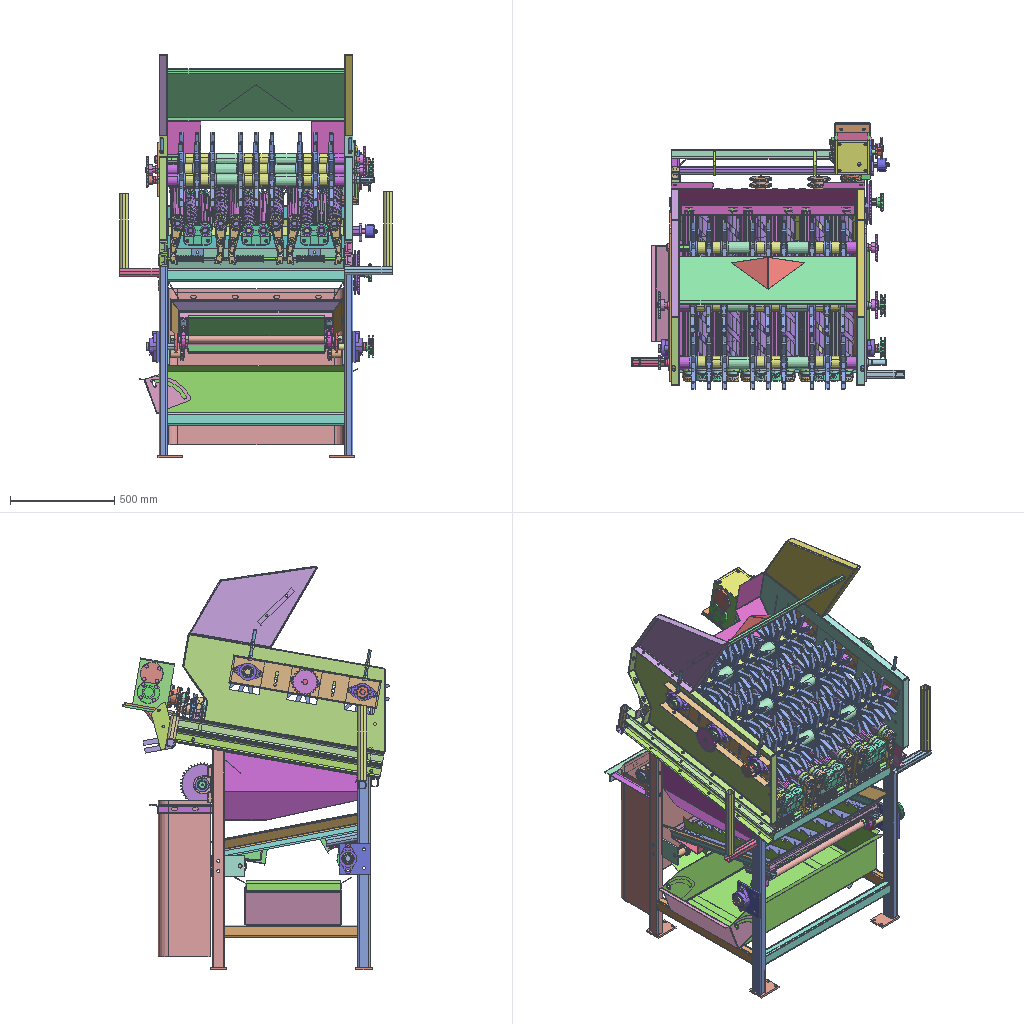Assembly | SolidWorks | 205 different items | 650 placed | box 1308 x 1283 x 1941 mm
Parts list (item | name | quantity | parent item | size | volume | features):
1 | (subassembly) | x2 | - | 262.006 x 262.006 x 1096 mm | 5906845 mm3 | features LayoutProfileFeature 1
2 | (subassembly) | x1 | in 3 | 32 x 32 x 1016 mm | 377179 mm3 | features LayoutProfileFeature 1
3 | (subassembly) | x1 | - | 262.006 x 262.006 x 1016 mm | 5789700 mm3 | features LayoutProfileFeature 1
4 | (subassembly) | x1 | - | 829.179 x 774.462 x 164.679 mm | 3231885 mm3 | features LayoutProfileFeature 1
5 | (subassembly) | x1 | in 6 | 1308 x 1116 x 1270 mm | 7450780 mm3 | features LayoutProfileFeature 1
6 | (subassembly) | x1 | - | 1308 x 1116 x 1280 mm | 8216576 mm3 | features LayoutProfileFeature 1
7 | (subassembly) | x1 | - | 1011 x 975.086 x 897.064 mm | 6794534 mm3 | features LayoutProfileFeature 1
8 | (subassembly) | x1 | in 7 | 852 x 259.795 x 223.71 mm | 531072 mm3 | features LayoutProfileFeature 1
9 | (subassembly) | x1 | - | - | 51530295 mm3 | features LayoutProfileFeature 1
10 | (subassembly) | x2 | in 7 | 136 x 720 x 55.5 mm | 917800 mm3 | features LayoutProfileFeature 1
11 | (subassembly) | x1 | in 43 | 5 x 8 x 18 mm | 644.24 mm3 | features LayoutProfileFeature 1
12 | (subassembly) | x1 | - | 95 x 60 x 141 mm | 156378 mm3 | features LayoutProfileFeature 1
13 | (subassembly) | x1 | - | 1048 x 561.923 x 252.092 mm | 2371643 mm3 | features LayoutProfileFeature 1
14 | (subassembly) | x2 | - | 171 x 100 x 85 mm | 236433 mm3 | features LayoutProfileFeature 1
15 | (subassembly) | x1 | in 24 | 680 x 740 x 40 mm | 649422 mm3 | features LayoutProfileFeature 1
16 | (subassembly) | x2 | in 1 | 32 x 32.7 x 1096 mm | 415799 mm3 | features LayoutProfileFeature 1
17 | (subassembly) | x1 | in 9 | 257.243 x 1277 x 974 mm | 4686993 mm3 | features LayoutProfileFeature 1
18 | (subassembly) | x2 | in 19 | 37 x 50 x 50 mm | 36117 mm3 | features LayoutProfileFeature 1
19 | (subassembly) | x1 | in 17 | 257.243 x 1277 x 974 mm | 4686993 mm3 | features LayoutProfileFeature 1
20 | (subassembly) | x6 | in 36 | - | 16373 mm3 | features LayoutProfileFeature 1
21 | (subassembly) | x12 | in 26, 30 | 60 x 226.322 x 40 mm | 177077 mm3 | features LayoutProfileFeature 1
22 | (subassembly) | x1 | in 43 | 5 x 8 x 18 mm | 644.24 mm3 | features LayoutProfileFeature 1
23 | (subassembly) | x2 | in 4 | 40 x 40 x 185 mm | 91393 mm3 | features LayoutProfileFeature 1
24 | (subassembly) | x1 | in 4 | 829.179 x 774.462 x 88.771 mm | 2637561 mm3 | features LayoutProfileFeature 1
25 | (subassembly) | x1 | - | 86.409 x 82.969 x 184 mm | 179233 mm3 | features LayoutProfileFeature 1
26 | (subassembly) | x3 | in 9 | 934.5 x 236.345 x 93.958 mm | 3556008 mm3 | features LayoutProfileFeature 1
27 | (subassembly) | x1 | in 5 | 932 x 40 x 300 mm | 437603 mm3 | features LayoutProfileFeature 1
28 | (subassembly) | x6 | in 26, 31, 34 | 926 x 69.689 x 69.689 mm | 3042926 mm3 | features LayoutProfileFeature 1
29 | (subassembly) | x3 | in 30 | 926 x 81.066 x 72.005 mm | 3183624 mm3 | features LayoutProfileFeature 1
30 | (subassembly) | x3 | in 9 | 934.5 x 238.062 x 84.273 mm | 3595919 mm3 | features LayoutProfileFeature 1
31 | (subassembly) | x1 | in 9 | 961.837 x 138.935 x 163.978 mm | 7248262 mm3 | features LayoutProfileFeature 1
32 | (subassembly) | x1 | in 31 | 955.318 x 72.003 x 80.734 mm | 3264645 mm3 | features LayoutProfileFeature 1
33 | (subassembly) | x1 | in 43 | 6 x 10 x 32 mm | 1765 mm3 | features LayoutProfileFeature 1
34 | (subassembly) | x2 | in 9 | 994 x 163.102 x 133.781 mm | 7441719 mm3 | features LayoutProfileFeature 1
35 | (subassembly) | x2 | in 34 | - | 3280765 mm3 | features LayoutProfileFeature 1
36 | (subassembly) | x6 | in 9 | 280 x 30 x 30 mm | 71173 mm3 | features LayoutProfileFeature 1
37 | (subassembly) | x2 | - | 64 x 64 x 86 mm | 122485 mm3 | features LayoutProfileFeature 1
38 | (subassembly) | x2 | - | - | 115965 mm3 | features LayoutProfileFeature 1
39 | (subassembly) | x2 | - | 49.4 x 172 x 90.1 mm | 253379 mm3 | features LayoutProfileFeature 1
40 | (subassembly) | x8 | in 10 | 142 x 52.5 x 83 mm | 159405 mm3 | features LayoutProfileFeature 1
41 | (subassembly) | x1 | in 15 | 680 x 740 x 40 mm | 324711 mm3 | features LayoutProfileFeature 1
42 | (subassembly) | x1 | in 43 | 246 x 230 x 166 mm | 1572970 mm3 | features LayoutProfileFeature 1
43 | (subassembly) | x1 | in 9 | 303.75 x 235 x 258.25 mm | 3389145 mm3 | features LayoutProfileFeature 1
44 | (subassembly) | x1 | in 25 | 5 x 8 x 28 mm | 1041 mm3 | features LayoutProfileFeature 1
45 | (subassembly) | x1 | in 43 | 7 x 8 x 25 mm | 1295 mm3 | features LayoutProfileFeature 1
46 | (subassembly) | x1 | in 43 | 7 x 8 x 28 mm | 1462 mm3 | features LayoutProfileFeature 1
47 | (subassembly) | x1 | in 43 | 8 x 10 x 40 mm | 2996 mm3 | features LayoutProfileFeature 1
48 | (subassembly) | x6 | in 31, 34 | 135 x 102.5 x 34.325 mm | 251519 mm3 | features LayoutProfileFeature 1
49 | - | x1 | in 43 | 7 x 52 x 52 mm | 5117 mm3 | features BaseBody 1
50 | - | x2 | in 5 | 40 x 60 x 928.577 mm | 490609 mm3 | features BaseBody 1
51 | - | x1 | in 5 | 40 x 63 x 1000 mm | 834296 mm3 | features BaseBody 1
52 | - | x1 | in 5 | 40 x 63 x 1000 mm | 834295 mm3 | features BaseBody 1
53 | - | x1 | - | 40 x 60 x 852 mm | 454199 mm3 | features BaseBody 1
54 | - | x4 | in 5 | 40 x 60 x 852 mm | 454199 mm3 | features BaseBody 1
55 | - | x2 | in 5 | 40 x 60 x 640 mm | 341182 mm3 | features BaseBody 1
56 | - | x4 | in 6 | 10 x 120 x 80 mm | 93345 mm3 | features BaseBody 1
57 | - | x2 | in 6 | 150 x 150 x 10 mm | 196208 mm3 | features BaseBody 1
58 | - | x1 | in 5 | 370 x 50 x 5 mm | 92500 mm3 | features BaseBody 1
59 | - | x2 | in 5, 19 | 60 x 150 x 12 mm | 89076 mm3 | features BaseBody 1
60 | - | x1 | in 43 | 7 x 40 x 40 mm | 2987 mm3 | features BaseBody 1
61 | - | x2 | in 27 | 40 x 40 x 260 mm | 77615 mm3 | features BaseBody 1
62 | - | x1 | in 27 | 40 x 40 x 932 mm | 282373 mm3 | features BaseBody 1
63 | - | x1 | in 5 | 40 x 40 x 188 mm | 95378 mm3 | features BaseBody 1
64 | - | x1 | in 5 | 40 x 40 x 228 mm | 115671 mm3 | features BaseBody 1
65 | - | x2 | in 5 | 40 x 40 x 360 mm | 182638 mm3 | features BaseBody 1
66 | - | x6 | in 28 | 767 x 69.535 x 69.535 mm | 2311745 mm3 | features CirPattern 1, Extrusion 1, ICE 1
67 | - | x24 | in 28, 29, 32, 35 | 17.5 x 67 x 67 mm | 46586 mm3 | features BaseBody 1
68 | - | x9 | in 28, 29 | 926 x 30 x 30 mm | 634773 mm3 | features BaseBody 1
69 | - | x2 | in 37 | 22 x 22 x 62 mm | 8301 mm3 | features BaseBody 1
70 | - | x6 | in 29, 32, 35 | - | - | features RefSurface 1
71 | - | x1 | in 43 | 7 x 50 x 50 mm | 4232 mm3 | features BaseBody 1
72 | - | x1 | in 12 | 137 x 32 x 32 mm | 102874 mm3 | features BaseBody 1
73 | - | x1 | in 43 | 243 x 32 x 32 mm | 178150 mm3 | features BaseBody 1
74 | - | x1 | in 43 | 175 x 35 x 35 mm | 112132 mm3 | features BaseBody 1
75 | - | x6 | in 36 | 280 x 16 x 16 mm | 51352 mm3 | features BaseBody 1
76 | - | x2 | in 35 | 987.5 x 30 x 30 mm | 660180 mm3 | features BaseBody 1
77 | - | x1 | in 32 | 955.3 x 30 x 30 mm | 646249 mm3 | features BaseBody 1
78 | - | x1 | in 43 | 10 x 100 x 100 mm | 37917 mm3 | features BaseBody 1
79 | - | x2 | in 12, 25 | 35 x 40 x 40 mm | 16618 mm3 | features BaseBody 1
80 | - | x1 | in 25 | 67.409 x 63.969 x 17.243 mm | 2142 mm3 | features BaseBody 3
81 | - | x1 | in 25 | 181 x 32 x 32 mm | 124690 mm3 | features BaseBody 1
82 | - | x1 | in 43 | 8 x 44.721 x 44.721 mm | 7123 mm3 | features BaseBody 1
83 | - | x2 | in 12, 25 | 95 x 60 x 10 mm | 34744 mm3 | features BaseBody 1
84 | - | x2 | in 39 | - | 74359 mm3 | features BaseBody 1
85 | - | x2 | in 14 | 85 x 35 x 35 mm | 67829 mm3 | features BaseBody 1
86 | - | x8 | in 40 | 142 x 34 x 83 mm | 116134 mm3 | features BaseBody 1
87 | - | x2 | in 38 | - | 77095 mm3 | features BaseBody 1
88 | - | x2 | in 39 | 48 x 172 x 90.1 mm | 179022 mm3 | features BaseBody 1
89 | - | x1 | in 43 | 64 x 115 x 115 mm | 164261 mm3 | features BaseBody 1
90 | - | x1 | in 2 | 32 x 79 x 32 mm | 51656 mm3 | features BaseBody 1
91 | - | x1 | - | 850 x 250 x 750 mm | 3902389 mm3 | features BaseBody 1
92 | - | x24 | in 28, 29, 32, 35 | 7 x 7 x 45 mm | 1727 mm3 | features BaseBody 1
93 | - | x1 | in 43 | 5 x 51.628 x 49.249 mm | 745.679 mm3 | features BaseBody 1
94 | - | x2 | in 43 | 97.808 x 97.316 x 49.456 mm | 114604 mm3 | features BaseBody 1
95 | - | x1 | - | 1048 x 561.923 x 252.092 mm | 2371643 mm3 | features BaseBody 4
96 | - | x2 | in 15, 41 | 40 x 40 x 740 mm | 169434 mm3 | features BaseBody 1
97 | - | x2 | in 15, 41 | 40 x 40 x 680 mm | 155277 mm3 | features BaseBody 1
98 | - | x18 | in 1, 3 | 60 x 40 x 60 mm | 62832 mm3 | features BaseBody 1
99 | - | x2 | in 43 | 95.704 x 96 x 20 mm | 90599 mm3 | features BaseBody 1
100 | - | x12 | in 26, 30, 31, 34 | 81.679 x 84 x 27 mm | 63908 mm3 | features BaseBody 1
101 | - | x5 | in 31, 34 | 105.504 x 105.504 x 30 mm | 102425 mm3 | features BaseBody 1
102 | - | x2 | in 10 | 136 x 720 x 43 mm | 439583 mm3 | features BaseBody 1
103 | - | x1 | in 43 | 23 x 110 x 110 mm | 98995 mm3 | features BaseBody 1
104 | - | x2 | in 14 | 35.48 x 38.644 x 1.2 mm | 408.802 mm3 | features BaseBody 1
105 | - | x1 | in 43 | 23 x 110 x 110 mm | 89416 mm3 | features BaseBody 1
106 | - | x1 | in 42 | 10 x 220 x 146 mm | 278281 mm3 | features BaseBody 1
107 | - | x2 | in 42 | 166 x 220 x 10 mm | 283430 mm3 | features BaseBody 1
108 | - | x1 | in 42 | 10 x 220 x 146 mm | 321200 mm3 | features BaseBody 1
109 | - | x1 | in 42 | 246 x 10 x 165 mm | 400376 mm3 | features BaseBody 1
110 | - | x1 | - | 825 x 35 x 35 mm | 733390 mm3 | features BaseBody 1
111 | - | x1 | in 43 | 230 x 30 x 30 mm | 136483 mm3 | features BaseBody 1
112 | - | x1 | - | 1025 x 40 x 40 mm | 1210935 mm3 | features BaseBody 1
113 | - | x20 | in 43 | 2.6 x 15.4 x 15.4 mm | 264.776 mm3 | features BaseBody 1
114 | - | x4 | in 43 | 2.1 x 12.3 x 12.3 mm | 137.595 mm3 | features BaseBody 1
115 | - | x1 | in 47 | 40 x 10 x 8 mm | 2996 mm3 | features BaseBody 1
116 | - | x1 | in 45 | 25 x 8 x 7 mm | 1295 mm3 | features BaseBody 1
117 | - | x2 | in 43 | 16.25 x 52 x 52 mm | 17643 mm3 | features BaseBody 2
118 | - | x1 | in 46 | 28 x 8 x 7 mm | 1462 mm3 | features BaseBody 1
119 | - | x1 | in 33 | 32 x 10 x 6 mm | 1765 mm3 | features BaseBody 1
120 | - | x2 | in 11, 22 | 18 x 8 x 5 mm | 644.24 mm3 | features BaseBody 1
121 | - | x1 | in 44 | 28 x 8 x 5 mm | 1041 mm3 | features BaseBody 1
122 | - | x4 | in 42 | 9.5 x 18.475 x 16 mm | 1563 mm3 | features BaseBody 1
123 | - | x4 | in 7 | 148.8 x 24.249 x 21 mm | 24876 mm3 | features BaseBody 1
124 | - | x8 | in 43 | 26.4 x 18.475 x 16 mm | 2940 mm3 | features BaseBody 1
125 | - | x12 | in 43 | 31.4 x 18.475 x 16 mm | 3333 mm3 | features BaseBody 1
126 | - | x4 | in 43 | 25.3 x 15.011 x 13 mm | 1747 mm3 | features BaseBody 1
127 | - | x2 | in 18 | 10.8 x 20.785 x 18 mm | 2091 mm3 | features BaseBody 1
128 | - | x4 | in 43 | 17.25 x 62 x 62 mm | 26692 mm3 | features BaseBody 2
129 | - | x2 | in 37 | 9.3 x 18.475 x 16 mm | 1467 mm3 | features BaseBody 1
130 | - | x12 | in 7 | 12 x 20.785 x 18 mm | 2327 mm3 | features BaseBody 1
131 | - | x2 | in 37 | 86 x 23.16 x 23.16 mm | 9538 mm3 | features BaseBody 1
132 | - | x2 | in 37 | 2 x 20 x 20 mm | 506.676 mm3 | features BaseBody 1
133 | - | x1 | - | 38.1 x 62 x 62 mm | 38870 mm3 | features BaseBody 1
134 | - | x10 | in 38, 40 | 38.1 x 62 x 62 mm | 38870 mm3 | features BaseBody 1
135 | - | x12 | in 26, 30, 31, 34 | 46 x 46 x 6 mm | 2288 mm3 | features BaseBody 1
136 | - | x1 | in 9 | 105.504 x 105.504 x 35 mm | 103891 mm3 | features BaseBody 1
137 | - | x6 | in 48 | 135 x 102.5 x 34.325 mm | 207829 mm3 | features BaseBody 1
138 | - | x1 | in 9 | 105.504 x 105.504 x 30 mm | 109846 mm3 | features BaseBody 1
139 | - | x1 | in 43 | 21 x 110 x 110 mm | 105066 mm3 | features BaseBody 1
140 | - | x12 | in 26, 30 | 22 x 22 x 80 mm | 22726 mm3 | features BaseBody 1
141 | - | x24 | in 26, 30, 31, 34 | 24 x 50 x 50 mm | 23661 mm3 | features BaseBody 1
142 | - | x1 | in 43 | 166 x 5 x 166 mm | 133883 mm3 | features BaseBody 1
143 | - | x1 | - | 22 x 22 x 80 mm | 22726 mm3 | features BaseBody 1
144 | - | x1 | in 7 | 181.421 x 291.421 x 932 mm | 492157 mm3 | features BaseBody 1
145 | - | x1 | - | 845 x 223.5 x 169.471 mm | 391233 mm3 | features BaseBody 1
146 | - | x1 | - | 845 x 40.182 x 116.821 mm | 185217 mm3 | features BaseBody 1
147 | - | x1 | in 19 | 40 x 63 x 1000 mm | 834296 mm3 | features BaseBody 1
148 | - | x1 | in 8 | 135.69 x 211.419 x 250.496 mm | 46324 mm3 | features BaseBody 1
149 | - | x1 | in 7 | 550.856 x 426.984 x 40 mm | 590475 mm3 | features BaseBody 1
150 | - | x1 | in 43 | 22 x 110 x 110 mm | 77102 mm3 | features BaseBody 1
151 | - | x1 | in 7 | 50 x 120 x 80 mm | 91955 mm3 | features BaseBody 1
152 | - | x1 | in 7 | 550.856 x 426.984 x 40 mm | 590475 mm3 | features BaseBody 1
153 | - | x1 | in 8 | 35.167 x 852 x 340.123 mm | 484748 mm3 | features BaseBody 1
154 | - | x1 | in 7 | 1030 x 400 x 40 mm | 1189266 mm3 | features BaseBody 1
155 | - | x1 | - | 640.37 x 331.413 x 119.799 mm | 282852 mm3 | features BaseBody 1
156 | - | x1 | in 13 | 1021 x 561.923 x 230 mm | 2027155 mm3 | features BaseBody 1
157 | - | x1 | in 13 | 465 x 201.23 x 182.5 mm | 260950 mm3 | features BaseBody 1
158 | - | x2 | in 13 | 31.5 x 460 x 31.5 mm | 41769 mm3 | features BaseBody 1
159 | - | x2 | in 14 | 160 x 100 x 10 mm | 144324 mm3 | features BaseBody 1
160 | - | x1 | in 43 | 100 x 100 x 1 mm | 4580 mm3 | features BaseBody 1
161 | - | x5 | in 1, 3 | 60 x 50 x 60 mm | 78540 mm3 | features BaseBody 1
162 | - | x1 | in 43 | 115 x 115 x 1 mm | 5935 mm3 | features BaseBody 1
163 | - | x2 | in 16 | 30 x 30 x 855 mm | 277.779 mm3 | features BaseBody 5
164 | - | x3 | in 2, 16 | 30 x 30 x 852 mm | 249719 mm3 | features BaseBody 1
165 | - | x3 | in 2, 16 | 32 x 123.5 x 32 mm | 75377 mm3 | features BaseBody 1
166 | - | x2 | in 16 | 32 x 158.5 x 32 mm | 90096 mm3 | features BaseBody 1
167 | - | x1 | in 2 | 30 x 30 x 855 mm | 282.424 mm3 | features BaseBody 5
168 | - | x2 | in 43 | 110 x 110 x 1 mm | 5272 mm3 | features BaseBody 1
169 | - | x12 | in 36 | 30 x 30 x 3 mm | 1722 mm3 | features BaseBody 1
170 | - | x1 | in 43 | 110 x 110 x 1 mm | 4275 mm3 | features BaseBody 1
171 | - | x27 | in 1, 3 | 264 x 35 x 264 mm | 515868 mm3 | features BaseBody 1
172 | - | x4 | in 37 | - | - | features RefSurface 7, BaseBody 2
173 | - | x1 | in 12 | 76 x 46 x 17.243 mm | 2142 mm3 | features BaseBody 3
174 | - | x1 | - | 211.077 x 210.652 x 26.852 mm | 750377 mm3 | features BaseBody 1
175 | - | x8 | in 40 | 38 x 38 x 10.3 mm | 4401 mm3 | features BaseBody 1
176 | - | x2 | in 37 | 64 x 64 x 42 mm | 76849 mm3 | features BaseBody 1
177 | - | x1 | - | 88.308 x 87.678 x 30 mm | 62261 mm3 | features BaseBody 1
178 | - | x3 | in 7 | 129.139 x 129.139 x 30 mm | 122850 mm3 | features BaseBody 1
179 | - | x2 | in 7, 9 | 66.851 x 66.851 x 30 mm | 34006 mm3 | features BaseBody 1
180 | - | x1 | in 7 | 1030 x 400 x 40 mm | 1189266 mm3 | features BaseBody 1
181 | - | x1 | - | 640.37 x 331.413 x 119.799 mm | 272644 mm3 | features BaseBody 1
182 | - | x2 | - | 107 x 107 x 35 mm | 157181 mm3 | features BaseBody 1
183 | - | x2 | in 14 | - | - | features RefSurface 9, BaseBody 2
184 | - | x1 | in 19 | 40 x 63 x 1000 mm | 834292 mm3 | features BaseBody 1
185 | - | x2 | in 18 | 37 x 50 x 50 mm | 34025 mm3 | features BaseBody 1
186 | - | x1 | in 19 | 170 x 277 x 10 mm | 446109 mm3 | features BaseBody 1
187 | - | x2 | in 19 | 80 x 215 x 10 mm | 139823 mm3 | features BaseBody 1
188 | - | x4 | in 19 | 60 x 40 x 10 mm | 22673 mm3 | features BaseBody 1
189 | - | x1 | in 19 | 40 x 40 x 185.969 mm | 74054 mm3 | features BaseBody 1
190 | - | x2 | in 19 | 852 x 14 x 60 mm | 682707 mm3 | features BaseBody 1
191 | - | x2 | in 19 | 40 x 40 x 111.5 mm | 56567 mm3 | features BaseBody 1
192 | - | x1 | in 19 | 40 x 40 x 962 mm | 488049 mm3 | features BaseBody 1
193 | - | x6 | in 20 | - | 16373 mm3 | features BaseBody 1
194 | - | x24 | in 21, 48 | 15 x 52 x 51.979 mm | 21846 mm3 | features BaseBody 1
195 | - | x12 | in 21 | 60 x 226.322 x 40 mm | 155209 mm3 | features BaseBody 1
196 | - | x2 | in 4 | 180 x 40 x 50 mm | 44356 mm3 | features BaseBody 1
197 | - | x2 | in 23 | 40 x 40 x 185 mm | 91393 mm3 | features BaseBody 1
198 | - | x2 | in 4 | 660 x 205.13 x 84 mm | 161412 mm3 | features BaseBody 1
199 | - | x1 | in 24 | 724 x 660 x 17 mm | 998776 mm3 | features BaseBody 1
200 | - | x6 | in 24 | 660 x 65 x 3 mm | 103950 mm3 | features BaseBody 1
201 | - | x2 | in 24 | 772 x 72.66 x 7.96 mm | 118787 mm3 | features BaseBody 1
202 | - | x1 | in 24 | 828 x 72.071 x 8.485 mm | 128085 mm3 | features BaseBody 1
203 | - | x1 | - | 1308 x 1116 x 1270 mm | 7450780 mm3 | features BaseBody 21
204 | - | x2 | in 5 | 40 x 60 x 1052 mm | 553157 mm3 | features BaseBody 1
205 | - | x6 | in 1, 3 | 60 x 100 x 60 mm | 157080 mm3 | features BaseBody 1
Mates (type | each side: item.copy, entity, surface, feature):
In the top assembly
Width | 61.1 face plane input 1 | 61.2 face plane input 1 | 91.1 face plane input 1 | 91.1 face plane input 1
Coincident | 62.1 face plane input 1 | 91.1 face plane input 1
Concentric | 174.1 face cylinder input 1 | 177.1 face cylinder input 1
Tangent | 52.1 face cylinder input 1 | 181.1 face plane input 1
Parallel | 52.1 face plane input 1 | 181.1 face plane input 1
Coincident | 52.1 face plane input 1 | 181.1 face plane input 1
DistanceDim | 50.1 edge | 181.1 face plane input 1
Width | 146.1 face plane input 1 | 146.1 face plane input 1 | 52.1 face plane input 1 | 51.1 face plane input 1
Concentric | 57.1 face cylinder input 1 | 86.1 face cylinder input 1 | 2 times
Concentric | 182.1 face cone input 1 | 175.1 face cylinder input 1
Coincident | 182.1 face plane input 1 | 175.1 face plane input 1
Concentric | 57.2 face cylinder input 1 | 86.2 face cylinder input 1 | 2 times
Coincident | 57.2 face plane input 1 | 86.2 face plane input 1
Coincident | 57.1 face plane input 1 | 86.1 face plane input 1
Coincident | 121.1 face plane input 1 | 182.1 face plane input 1
Coincident | 204.1 face plane input 1 | 159.1 face plane input 1
Slot | 204.1 face cylinder input 1 | 159.1 face plane input 1 | 2 times
Coincident | 204.2 face plane input 1 | 159.2 face plane input 1 | 2 times
Concentric | 159.2 face cylinder input 1 | 159.1 face cylinder input 1 | 2 times
Coincident | 87.1 face plane input 1 | 197.1 face plane input 1
Coincident | 87.2 face plane input 1 | 197.2 face plane input 1
Tangent | 87.2 face plane input 1 | 197.2 face cylinder input 1
Parallel | 87.1 face plane input 1 | 197.1 face plane input 1 | 2 times
Concentric | 87.1 face cylinder input 1 | 197.1 face cylinder input 1
Tangent | 183.1 face cylinder input 2 | 196.1 face plane input 1
Tangent | 204.2 face cylinder input 1 | 159.2 face plane input 1
Parallel | 204.2 face plane input 1 | 159.2 face plane input 1
Concentric | 81.1 face cylinder input 1 | 182.1 face cylinder input 1
Concentric | 79.1 face cylinder input 1 | 110.1 face cylinder input 1
Coincident | 79.1 face plane input 1 | 110.1 face plane input 1
Coincident | 81.1 face plane input 1 | 182.1 face plane input 1
Concentric | 134.1 face cylinder input 1 | 110.1 face cylinder input 1
Concentric | 87.2 face cylinder input 1 | 197.2 face cylinder input 1
Coincident | 134.1 face plane input 1 | 110.1 face plane input 1
Parallel | 87.1 face plane input 1 | 87.2 face plane input 1
Width | 87.1 face plane input 1 | 87.1 face plane input 1 | 197.1 face plane input 1 | 197.1 face plane input 1
Concentric | 79.2 face cylinder input 1 | 110.1 face cylinder input 1
Coincident | 79.2 face plane input 1 | 110.1 face plane input 1
Concentric | 72.1 face cylinder input 1 | 175.2 face cylinder input 1
Concentric | 204.1 face cylinder input 1 | 88.1 face cylinder input 1
Parallel | 204.1 face plane input 1 | 88.1 face plane input 1
Concentric | 84.1 face cylinder input 1 | 84.2 face cylinder input 1
DistanceDim | 88.2 face plane input 1 | 204.2 face plane input 1
Concentric | 112.1 face cylinder input 1 | 84.1 face cylinder input 1
Concentric | 112.1 face cylinder input 1 | 177.1 face cylinder input 1
Concentric | 112.1 face cylinder input 1 | 174.1 face cylinder input 1
Coincident | 112.1 face plane input 1 | 174.1 face plane input 1
Coincident | 84.1 face plane input 1 | 174.1 face plane input 1
Coincident | 112.1 face plane input 1 | 177.1 face plane input 1 | 2 times
Coincident | 204.2 face plane input 1 | 88.2 face plane input 1
Coincident | 112.1 face plane input 1 | 84.2 face plane input 1
Concentric | 85.1 face cylinder input 1 | 85.2 face cylinder input 1
DistanceDim | 159.1 face plane input 1 | 204.1 face plane input 1
Concentric | 52.1 face cylinder input 1 | 184.1 face cylinder input 1 | 2 times
Coincident | 52.1 face plane input 1 | 184.1 face plane input 1
Concentric | 184.1 face cylinder input 1 | 180.1 face cylinder input 1 | 2 times
Coincident | 184.1 face plane input 1 | 180.1 face plane input 1
Concentric | 175.3 edge | 166.1 face cylinder input 1
Coincident | 102.1 face plane input 1 | 161.1 face plane input 1
Concentric | 175.4 face cylinder input 1 | 166.2 face cylinder input 1
Coincident | 180.1 face plane input 1 | 161.2 face plane input 1
Concentric | 178.1 face cylinder input 1 | 166.2 face cylinder input 1
Concentric | 182.2 face cylinder input 1 | 166.2 face cylinder input 1
Coincident | 178.1 face plane input 1 | 166.2 face plane input 1
Parallel | 178.1 face plane input 1 | 166.2 face plane input 1
Coincident | 182.2 face plane input 1 | 178.1 face plane input 1
Coincident | 182.2 face plane input 1 | 166.2 face plane input 1
Concentric | 175.5 face cylinder input 1 | 165.1 face cylinder input 1
Coincident | 102.1 face plane input 1 | 161.3 face plane input 1
Concentric | 165.1 face cylinder input 1 | 178.2 face cylinder input 1
Coincident | 165.1 face plane input 1 | 178.2 face plane input 1
Coincident | 178.1 face plane input 1 | 178.2 face plane input 1
In subassembly 14
Concentric | 85.3 face cylinder input 1 | 183.2 face cylinder input 1
Concentric | 159.3 face cylinder input 1 | 85.3 face cylinder input 1
Concentric | 183.2 face cylinder input 1 | 104.1 face cylinder input 1
Coincident | 85.3 face plane input 1 | 183.2 face plane input 1
Coincident | 183.2 face plane input 1 | 104.1 face plane input 1
Coincident | 159.3 face plane input 1 | 85.3 face plane input 1
In subassembly 25
Concentric | 81.2 face cylinder input 1 | 83.1 face cylinder input 1
Coincident | 81.2 face plane input 1 | 121.2 face plane input 1 | 2 times
Concentric | 81.2 face cylinder input 1 | 121.2 face cylinder input 1
Concentric | 83.1 face cylinder input 1 | 79.3 face cylinder input 1
Coincident | 83.1 face plane input 1 | 79.3 face plane input 1
Concentric | 80.1 face cylinder input 1 | 79.3 face cylinder input 1
Concentric | 80.1 face cone input 1 | 81.2 face cylinder input 1
Coincident | 80.1 face plane input 3 | 83.1 face plane input 1
Coincident | 81.2 face plane input 1 | 83.1 face plane input 1